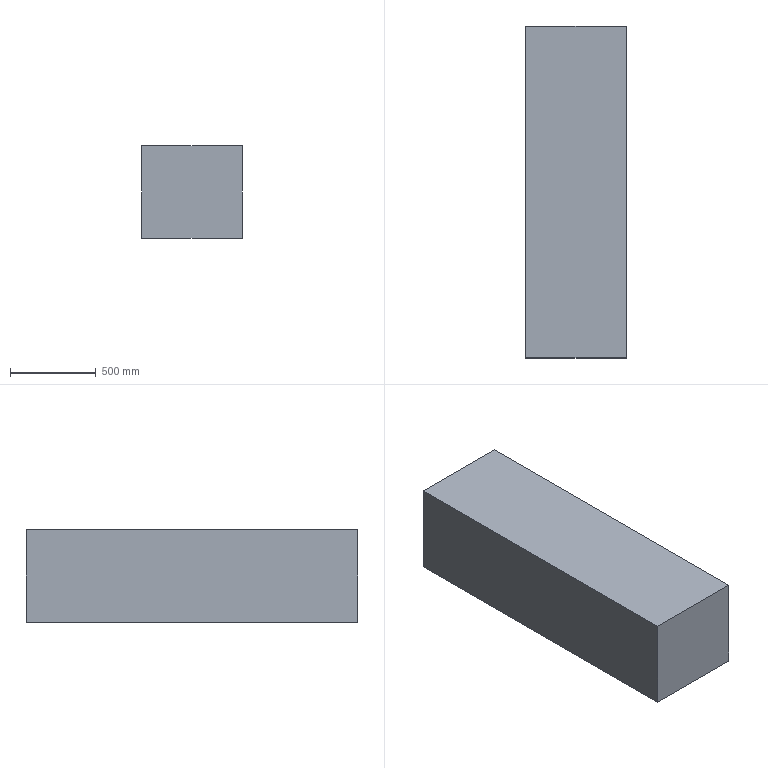Part | STEP file | WORK.1.stp | 1 solid | 6 faces | box 587 x 1931 x 541 mm | volume 613221877 mm3 | plane 6
STEP:
#1=CARTESIAN_POINT('',(0.,0.,0.));
#2=DIRECTION('',(0.,0.,1.));
#3=DIRECTION('',(1.,0.,0.));
#4=AXIS2_PLACEMENT_3D('',#1,#2,#3);
#5=CARTESIAN_POINT('',(293.5,965.5,-270.5));
#6=VERTEX_POINT('',#5);
#7=CARTESIAN_POINT('',(-293.5,965.5,-270.5));
#8=VERTEX_POINT('',#7);
#9=CARTESIAN_POINT('',(293.5,965.5,-270.5));
#10=DIRECTION('',(-1.,0.,0.));
#11=VECTOR('',#10,1.);
#12=LINE('',#9,#11);
#13=CARTESIAN_POINT('',(0.,965.5,0.));
#14=DIRECTION('',(0.,-1.,0.));
#15=DIRECTION('',(0.,0.,-1.));
#16=AXIS2_PLACEMENT_3D('',#13,#14,#15);
#17=PLANE('',#16);
#18=CARTESIAN_POINT('',(270.5,293.5));
#19=DIRECTION('',(0.,-1.));
#20=VECTOR('',#19,1.);
#21=LINE('',#18,#20);
#22=(GEOMETRIC_REPRESENTATION_CONTEXT(2)PARAMETRIC_REPRESENTATION_CONTEXT()REPRESENTATION_CONTEXT('',''));
#23=DEFINITIONAL_REPRESENTATION('',(#21),#22);
#24=PCURVE('',#17,#23);
#25=CARTESIAN_POINT('',(0.,0.,-270.5));
#26=DIRECTION('',(0.,0.,1.));
#27=DIRECTION('',(1.,0.,0.));
#28=AXIS2_PLACEMENT_3D('',#25,#26,#27);
#29=PLANE('',#28);
#30=CARTESIAN_POINT('',(293.5,965.5));
#31=DIRECTION('',(-1.,0.));
#32=VECTOR('',#31,1.);
#33=LINE('',#30,#32);
#34=(GEOMETRIC_REPRESENTATION_CONTEXT(2)PARAMETRIC_REPRESENTATION_CONTEXT()REPRESENTATION_CONTEXT('',''));
#35=DEFINITIONAL_REPRESENTATION('',(#33),#34);
#36=PCURVE('',#29,#35);
#37=SURFACE_CURVE('',#12,(#24,#36),.PCURVE_S1.);
#38=EDGE_CURVE('',#6,#8,#37,.T.);
#39=ORIENTED_EDGE('',*,*,#38,.T.);
#40=CARTESIAN_POINT('',(-293.5,965.5,270.5));
#41=VERTEX_POINT('',#40);
#42=CARTESIAN_POINT('',(-293.5,965.5,270.5));
#43=DIRECTION('',(0.,0.,-1.));
#44=VECTOR('',#43,1.);
#45=LINE('',#42,#44);
#46=CARTESIAN_POINT('',(-270.5,-293.5));
#47=DIRECTION('',(1.,0.));
#48=VECTOR('',#47,1.);
#49=LINE('',#46,#48);
#50=(GEOMETRIC_REPRESENTATION_CONTEXT(2)PARAMETRIC_REPRESENTATION_CONTEXT()REPRESENTATION_CONTEXT('',''));
#51=DEFINITIONAL_REPRESENTATION('',(#49),#50);
#52=PCURVE('',#17,#51);
#53=CARTESIAN_POINT('',(-293.5,0.,0.));
#54=DIRECTION('',(1.,0.,0.));
#55=DIRECTION('',(0.,1.,0.));
#56=AXIS2_PLACEMENT_3D('',#53,#54,#55);
#57=PLANE('',#56);
#58=CARTESIAN_POINT('',(965.5,270.5));
#59=DIRECTION('',(0.,-1.));
#60=VECTOR('',#59,1.);
#61=LINE('',#58,#60);
#62=(GEOMETRIC_REPRESENTATION_CONTEXT(2)PARAMETRIC_REPRESENTATION_CONTEXT()REPRESENTATION_CONTEXT('',''));
#63=DEFINITIONAL_REPRESENTATION('',(#61),#62);
#64=PCURVE('',#57,#63);
#65=SURFACE_CURVE('',#45,(#52,#64),.PCURVE_S1.);
#66=EDGE_CURVE('',#41,#8,#65,.T.);
#67=ORIENTED_EDGE('',*,*,#66,.F.);
#68=CARTESIAN_POINT('',(293.5,965.5,270.5));
#69=VERTEX_POINT('',#68);
#70=CARTESIAN_POINT('',(293.5,965.5,270.5));
#71=DIRECTION('',(-1.,0.,0.));
#72=VECTOR('',#71,1.);
#73=LINE('',#70,#72);
#74=CARTESIAN_POINT('',(-270.5,293.5));
#75=DIRECTION('',(0.,-1.));
#76=VECTOR('',#75,1.);
#77=LINE('',#74,#76);
#78=(GEOMETRIC_REPRESENTATION_CONTEXT(2)PARAMETRIC_REPRESENTATION_CONTEXT()REPRESENTATION_CONTEXT('',''));
#79=DEFINITIONAL_REPRESENTATION('',(#77),#78);
#80=PCURVE('',#17,#79);
#81=CARTESIAN_POINT('',(0.,0.,270.5));
#82=DIRECTION('',(0.,0.,-1.));
#83=DIRECTION('',(0.,-1.,0.));
#84=AXIS2_PLACEMENT_3D('',#81,#82,#83);
#85=PLANE('',#84);
#86=CARTESIAN_POINT('',(-965.5,-293.5));
#87=DIRECTION('',(0.,1.));
#88=VECTOR('',#87,1.);
#89=LINE('',#86,#88);
#90=(GEOMETRIC_REPRESENTATION_CONTEXT(2)PARAMETRIC_REPRESENTATION_CONTEXT()REPRESENTATION_CONTEXT('',''));
#91=DEFINITIONAL_REPRESENTATION('',(#89),#90);
#92=PCURVE('',#85,#91);
#93=SURFACE_CURVE('',#73,(#80,#92),.PCURVE_S1.);
#94=EDGE_CURVE('',#69,#41,#93,.T.);
#95=ORIENTED_EDGE('',*,*,#94,.F.);
#96=CARTESIAN_POINT('',(293.5,965.5,-270.5));
#97=DIRECTION('',(0.,0.,1.));
#98=VECTOR('',#97,1.);
#99=LINE('',#96,#98);
#100=CARTESIAN_POINT('',(270.5,293.5));
#101=DIRECTION('',(-1.,0.));
#102=VECTOR('',#101,1.);
#103=LINE('',#100,#102);
#104=(GEOMETRIC_REPRESENTATION_CONTEXT(2)PARAMETRIC_REPRESENTATION_CONTEXT()REPRESENTATION_CONTEXT('',''));
#105=DEFINITIONAL_REPRESENTATION('',(#103),#104);
#106=PCURVE('',#17,#105);
#107=CARTESIAN_POINT('',(293.5,0.,0.));
#108=DIRECTION('',(1.,0.,0.));
#109=DIRECTION('',(0.,1.,0.));
#110=AXIS2_PLACEMENT_3D('',#107,#108,#109);
#111=PLANE('',#110);
#112=CARTESIAN_POINT('',(965.5,-270.5));
#113=DIRECTION('',(0.,1.));
#114=VECTOR('',#113,1.);
#115=LINE('',#112,#114);
#116=(GEOMETRIC_REPRESENTATION_CONTEXT(2)PARAMETRIC_REPRESENTATION_CONTEXT()REPRESENTATION_CONTEXT('',''));
#117=DEFINITIONAL_REPRESENTATION('',(#115),#116);
#118=PCURVE('',#111,#117);
#119=SURFACE_CURVE('',#99,(#106,#118),.PCURVE_S1.);
#120=EDGE_CURVE('',#6,#69,#119,.T.);
#121=ORIENTED_EDGE('',*,*,#120,.F.);
#122=EDGE_LOOP('',(#39,#67,#95,#121));
#123=FACE_BOUND('',#122,.T.);
#124=ADVANCED_FACE('',(#123),#17,.F.);
#125=ORIENTED_EDGE('',*,*,#94,.T.);
#126=CARTESIAN_POINT('',(-293.5,-965.5,270.5));
#127=VERTEX_POINT('',#126);
#128=CARTESIAN_POINT('',(-293.5,-965.5,270.5));
#129=DIRECTION('',(0.,1.,0.));
#130=VECTOR('',#129,1.);
#131=LINE('',#128,#130);
#132=CARTESIAN_POINT('',(965.5,293.5));
#133=DIRECTION('',(-1.,0.));
#134=VECTOR('',#133,1.);
#135=LINE('',#132,#134);
#136=(GEOMETRIC_REPRESENTATION_CONTEXT(2)PARAMETRIC_REPRESENTATION_CONTEXT()REPRESENTATION_CONTEXT('',''));
#137=DEFINITIONAL_REPRESENTATION('',(#135),#136);
#138=PCURVE('',#85,#137);
#139=CARTESIAN_POINT('',(-965.5,270.5));
#140=DIRECTION('',(1.,0.));
#141=VECTOR('',#140,1.);
#142=LINE('',#139,#141);
#143=(GEOMETRIC_REPRESENTATION_CONTEXT(2)PARAMETRIC_REPRESENTATION_CONTEXT()REPRESENTATION_CONTEXT('',''));
#144=DEFINITIONAL_REPRESENTATION('',(#142),#143);
#145=PCURVE('',#57,#144);
#146=SURFACE_CURVE('',#131,(#138,#145),.PCURVE_S1.);
#147=EDGE_CURVE('',#127,#41,#146,.T.);
#148=ORIENTED_EDGE('',*,*,#147,.F.);
#149=CARTESIAN_POINT('',(293.5,-965.5,270.5));
#150=VERTEX_POINT('',#149);
#151=CARTESIAN_POINT('',(293.5,-965.5,270.5));
#152=DIRECTION('',(-1.,0.,0.));
#153=VECTOR('',#152,1.);
#154=LINE('',#151,#153);
#155=CARTESIAN_POINT('',(965.5,-293.5));
#156=DIRECTION('',(0.,1.));
#157=VECTOR('',#156,1.);
#158=LINE('',#155,#157);
#159=(GEOMETRIC_REPRESENTATION_CONTEXT(2)PARAMETRIC_REPRESENTATION_CONTEXT()REPRESENTATION_CONTEXT('',''));
#160=DEFINITIONAL_REPRESENTATION('',(#158),#159);
#161=PCURVE('',#85,#160);
#162=CARTESIAN_POINT('',(0.,-965.5,0.));
#163=DIRECTION('',(0.,1.,0.));
#164=DIRECTION('',(1.,0.,0.));
#165=AXIS2_PLACEMENT_3D('',#162,#163,#164);
#166=PLANE('',#165);
#167=CARTESIAN_POINT('',(293.5,-270.5));
#168=DIRECTION('',(-1.,0.));
#169=VECTOR('',#168,1.);
#170=LINE('',#167,#169);
#171=(GEOMETRIC_REPRESENTATION_CONTEXT(2)PARAMETRIC_REPRESENTATION_CONTEXT()REPRESENTATION_CONTEXT('',''));
#172=DEFINITIONAL_REPRESENTATION('',(#170),#171);
#173=PCURVE('',#166,#172);
#174=SURFACE_CURVE('',#154,(#161,#173),.PCURVE_S1.);
#175=EDGE_CURVE('',#150,#127,#174,.T.);
#176=ORIENTED_EDGE('',*,*,#175,.F.);
#177=CARTESIAN_POINT('',(293.5,965.5,270.5));
#178=DIRECTION('',(0.,-1.,0.));
#179=VECTOR('',#178,1.);
#180=LINE('',#177,#179);
#181=CARTESIAN_POINT('',(-965.5,-293.5));
#182=DIRECTION('',(1.,0.));
#183=VECTOR('',#182,1.);
#184=LINE('',#181,#183);
#185=(GEOMETRIC_REPRESENTATION_CONTEXT(2)PARAMETRIC_REPRESENTATION_CONTEXT()REPRESENTATION_CONTEXT('',''));
#186=DEFINITIONAL_REPRESENTATION('',(#184),#185);
#187=PCURVE('',#85,#186);
#188=CARTESIAN_POINT('',(965.5,270.5));
#189=DIRECTION('',(-1.,0.));
#190=VECTOR('',#189,1.);
#191=LINE('',#188,#190);
#192=(GEOMETRIC_REPRESENTATION_CONTEXT(2)PARAMETRIC_REPRESENTATION_CONTEXT()REPRESENTATION_CONTEXT('',''));
#193=DEFINITIONAL_REPRESENTATION('',(#191),#192);
#194=PCURVE('',#111,#193);
#195=SURFACE_CURVE('',#180,(#187,#194),.PCURVE_S1.);
#196=EDGE_CURVE('',#69,#150,#195,.T.);
#197=ORIENTED_EDGE('',*,*,#196,.F.);
#198=EDGE_LOOP('',(#125,#148,#176,#197));
#199=FACE_BOUND('',#198,.T.);
#200=ADVANCED_FACE('',(#199),#85,.F.);
#201=ORIENTED_EDGE('',*,*,#175,.T.);
#202=CARTESIAN_POINT('',(-293.5,-965.5,-270.5));
#203=VERTEX_POINT('',#202);
#204=CARTESIAN_POINT('',(-293.5,-965.5,-270.5));
#205=DIRECTION('',(0.,0.,1.));
#206=VECTOR('',#205,1.);
#207=LINE('',#204,#206);
#208=CARTESIAN_POINT('',(-293.5,270.5));
#209=DIRECTION('',(0.,-1.));
#210=VECTOR('',#209,1.);
#211=LINE('',#208,#210);
#212=(GEOMETRIC_REPRESENTATION_CONTEXT(2)PARAMETRIC_REPRESENTATION_CONTEXT()REPRESENTATION_CONTEXT('',''));
#213=DEFINITIONAL_REPRESENTATION('',(#211),#212);
#214=PCURVE('',#166,#213);
#215=CARTESIAN_POINT('',(-965.5,-270.5));
#216=DIRECTION('',(0.,1.));
#217=VECTOR('',#216,1.);
#218=LINE('',#215,#217);
#219=(GEOMETRIC_REPRESENTATION_CONTEXT(2)PARAMETRIC_REPRESENTATION_CONTEXT()REPRESENTATION_CONTEXT('',''));
#220=DEFINITIONAL_REPRESENTATION('',(#218),#219);
#221=PCURVE('',#57,#220);
#222=SURFACE_CURVE('',#207,(#214,#221),.PCURVE_S1.);
#223=EDGE_CURVE('',#203,#127,#222,.T.);
#224=ORIENTED_EDGE('',*,*,#223,.F.);
#225=CARTESIAN_POINT('',(293.5,-965.5,-270.5));
#226=VERTEX_POINT('',#225);
#227=CARTESIAN_POINT('',(293.5,-965.5,-270.5));
#228=DIRECTION('',(-1.,0.,0.));
#229=VECTOR('',#228,1.);
#230=LINE('',#227,#229);
#231=CARTESIAN_POINT('',(293.5,270.5));
#232=DIRECTION('',(-1.,0.));
#233=VECTOR('',#232,1.);
#234=LINE('',#231,#233);
#235=(GEOMETRIC_REPRESENTATION_CONTEXT(2)PARAMETRIC_REPRESENTATION_CONTEXT()REPRESENTATION_CONTEXT('',''));
#236=DEFINITIONAL_REPRESENTATION('',(#234),#235);
#237=PCURVE('',#166,#236);
#238=CARTESIAN_POINT('',(293.5,-965.5));
#239=DIRECTION('',(-1.,0.));
#240=VECTOR('',#239,1.);
#241=LINE('',#238,#240);
#242=(GEOMETRIC_REPRESENTATION_CONTEXT(2)PARAMETRIC_REPRESENTATION_CONTEXT()REPRESENTATION_CONTEXT('',''));
#243=DEFINITIONAL_REPRESENTATION('',(#241),#242);
#244=PCURVE('',#29,#243);
#245=SURFACE_CURVE('',#230,(#237,#244),.PCURVE_S1.);
#246=EDGE_CURVE('',#226,#203,#245,.T.);
#247=ORIENTED_EDGE('',*,*,#246,.F.);
#248=CARTESIAN_POINT('',(293.5,-965.5,270.5));
#249=DIRECTION('',(0.,0.,-1.));
#250=VECTOR('',#249,1.);
#251=LINE('',#248,#250);
#252=CARTESIAN_POINT('',(293.5,-270.5));
#253=DIRECTION('',(0.,1.));
#254=VECTOR('',#253,1.);
#255=LINE('',#252,#254);
#256=(GEOMETRIC_REPRESENTATION_CONTEXT(2)PARAMETRIC_REPRESENTATION_CONTEXT()REPRESENTATION_CONTEXT('',''));
#257=DEFINITIONAL_REPRESENTATION('',(#255),#256);
#258=PCURVE('',#166,#257);
#259=CARTESIAN_POINT('',(-965.5,270.5));
#260=DIRECTION('',(0.,-1.));
#261=VECTOR('',#260,1.);
#262=LINE('',#259,#261);
#263=(GEOMETRIC_REPRESENTATION_CONTEXT(2)PARAMETRIC_REPRESENTATION_CONTEXT()REPRESENTATION_CONTEXT('',''));
#264=DEFINITIONAL_REPRESENTATION('',(#262),#263);
#265=PCURVE('',#111,#264);
#266=SURFACE_CURVE('',#251,(#258,#265),.PCURVE_S1.);
#267=EDGE_CURVE('',#150,#226,#266,.T.);
#268=ORIENTED_EDGE('',*,*,#267,.F.);
#269=EDGE_LOOP('',(#201,#224,#247,#268));
#270=FACE_BOUND('',#269,.T.);
#271=ADVANCED_FACE('',(#270),#166,.F.);
#272=ORIENTED_EDGE('',*,*,#246,.T.);
#273=CARTESIAN_POINT('',(-293.5,965.5,-270.5));
#274=DIRECTION('',(0.,-1.,0.));
#275=VECTOR('',#274,1.);
#276=LINE('',#273,#275);
#277=CARTESIAN_POINT('',(-293.5,965.5));
#278=DIRECTION('',(0.,-1.));
#279=VECTOR('',#278,1.);
#280=LINE('',#277,#279);
#281=(GEOMETRIC_REPRESENTATION_CONTEXT(2)PARAMETRIC_REPRESENTATION_CONTEXT()REPRESENTATION_CONTEXT('',''));
#282=DEFINITIONAL_REPRESENTATION('',(#280),#281);
#283=PCURVE('',#29,#282);
#284=CARTESIAN_POINT('',(965.5,-270.5));
#285=DIRECTION('',(-1.,0.));
#286=VECTOR('',#285,1.);
#287=LINE('',#284,#286);
#288=(GEOMETRIC_REPRESENTATION_CONTEXT(2)PARAMETRIC_REPRESENTATION_CONTEXT()REPRESENTATION_CONTEXT('',''));
#289=DEFINITIONAL_REPRESENTATION('',(#287),#288);
#290=PCURVE('',#57,#289);
#291=SURFACE_CURVE('',#276,(#283,#290),.PCURVE_S1.);
#292=EDGE_CURVE('',#8,#203,#291,.T.);
#293=ORIENTED_EDGE('',*,*,#292,.F.);
#294=ORIENTED_EDGE('',*,*,#38,.F.);
#295=CARTESIAN_POINT('',(293.5,-965.5,-270.5));
#296=DIRECTION('',(0.,1.,0.));
#297=VECTOR('',#296,1.);
#298=LINE('',#295,#297);
#299=CARTESIAN_POINT('',(293.5,-965.5));
#300=DIRECTION('',(0.,1.));
#301=VECTOR('',#300,1.);
#302=LINE('',#299,#301);
#303=(GEOMETRIC_REPRESENTATION_CONTEXT(2)PARAMETRIC_REPRESENTATION_CONTEXT()REPRESENTATION_CONTEXT('',''));
#304=DEFINITIONAL_REPRESENTATION('',(#302),#303);
#305=PCURVE('',#29,#304);
#306=CARTESIAN_POINT('',(-965.5,-270.5));
#307=DIRECTION('',(1.,0.));
#308=VECTOR('',#307,1.);
#309=LINE('',#306,#308);
#310=(GEOMETRIC_REPRESENTATION_CONTEXT(2)PARAMETRIC_REPRESENTATION_CONTEXT()REPRESENTATION_CONTEXT('',''));
#311=DEFINITIONAL_REPRESENTATION('',(#309),#310);
#312=PCURVE('',#111,#311);
#313=SURFACE_CURVE('',#298,(#305,#312),.PCURVE_S1.);
#314=EDGE_CURVE('',#226,#6,#313,.T.);
#315=ORIENTED_EDGE('',*,*,#314,.F.);
#316=EDGE_LOOP('',(#272,#293,#294,#315));
#317=FACE_BOUND('',#316,.T.);
#318=ADVANCED_FACE('',(#317),#29,.F.);
#319=ORIENTED_EDGE('',*,*,#66,.T.);
#320=ORIENTED_EDGE('',*,*,#292,.T.);
#321=ORIENTED_EDGE('',*,*,#223,.T.);
#322=ORIENTED_EDGE('',*,*,#147,.T.);
#323=EDGE_LOOP('',(#319,#320,#321,#322));
#324=FACE_BOUND('',#323,.T.);
#325=ADVANCED_FACE('',(#324),#57,.F.);
#326=ORIENTED_EDGE('',*,*,#120,.T.);
#327=ORIENTED_EDGE('',*,*,#196,.T.);
#328=ORIENTED_EDGE('',*,*,#267,.T.);
#329=ORIENTED_EDGE('',*,*,#314,.T.);
#330=EDGE_LOOP('',(#326,#327,#328,#329));
#331=FACE_BOUND('',#330,.T.);
#332=ADVANCED_FACE('',(#331),#111,.T.);
#333=CLOSED_SHELL('',(#124,#200,#271,#318,#325,#332));
#334=MANIFOLD_SOLID_BREP('',#333);
#335=(LENGTH_UNIT()NAMED_UNIT(*)SI_UNIT(.MILLI.,.METRE.));
#336=UNCERTAINTY_MEASURE_WITH_UNIT(LENGTH_MEASURE(0.0000001),#335,'','');
#337=(NAMED_UNIT(*)PLANE_ANGLE_UNIT()SI_UNIT($,.RADIAN.));
#338=(NAMED_UNIT(*)SI_UNIT($,.STERADIAN.)SOLID_ANGLE_UNIT());
#339=(GEOMETRIC_REPRESENTATION_CONTEXT(3)GLOBAL_UNCERTAINTY_ASSIGNED_CONTEXT((#336))GLOBAL_UNIT_ASSIGNED_CONTEXT((#335,#337,#338))REPRESENTATION_CONTEXT('',''));
#340=ADVANCED_BREP_SHAPE_REPRESENTATION('',(#4,#334),#339);